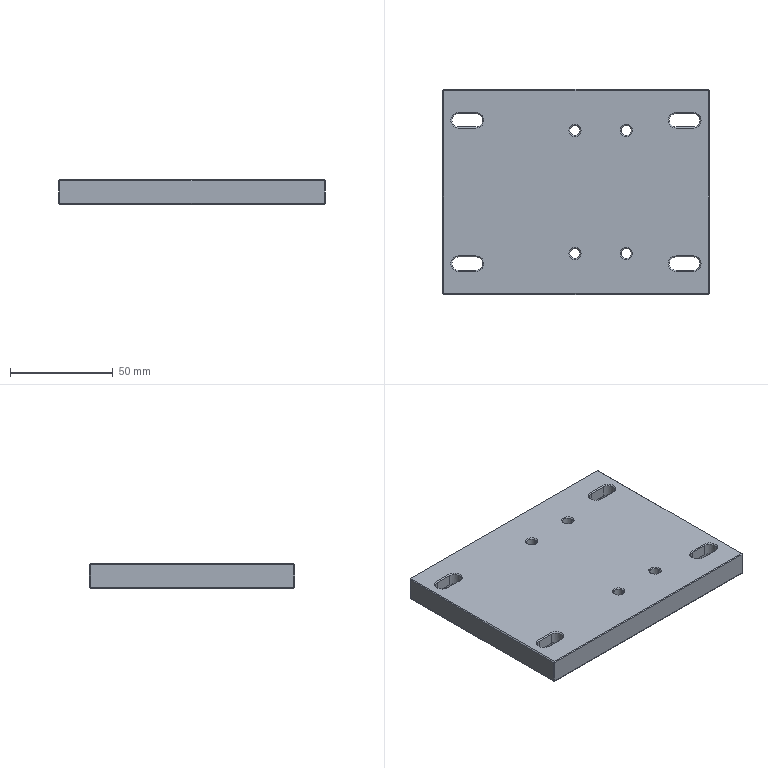Part | SolidWorks | features HoleWzd 2, Chamfer 1, Extrusion 1 | 1 solid | 134 faces | box 130 x 100 x 12 mm | volume 148225 mm3 | plane 62 | cone 40 | cylinder 32 | commonest cylinder face diameters 6.6 x12 11 x12 5 x8